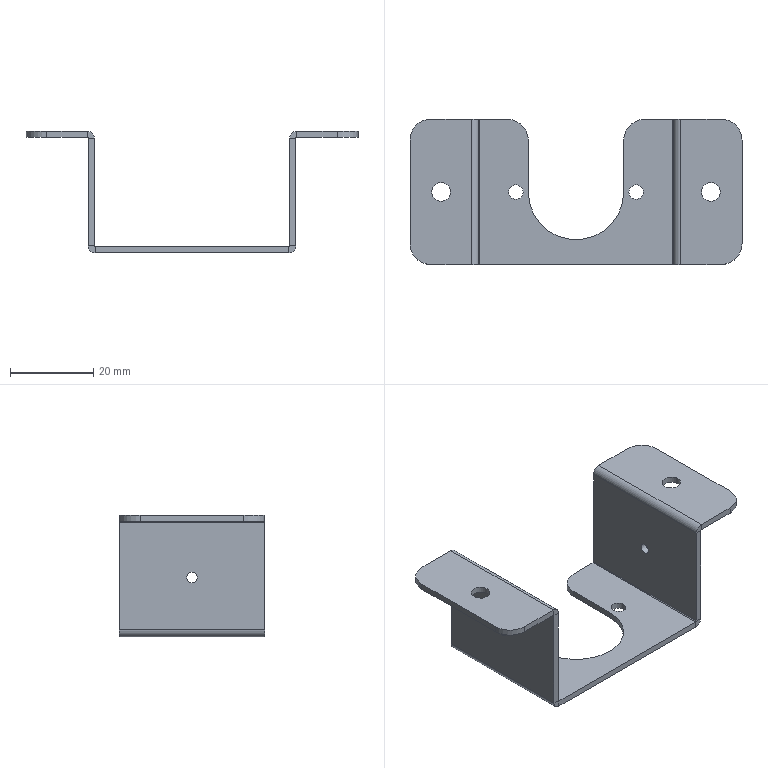Part | NX | 1 solid | 54 faces | box 80 x 35 x 29.3 mm | volume 5978 mm3 | plane 33 | cylinder 21 | commonest cylinder face diameters 10 x6 0.4 x4 3.4 x4 2.5 x2 3.5 x2 4.5 x2
STEP:
#1=CARTESIAN_POINT('',(-12.75,0.,-1.5));
#2=VERTEX_POINT('',#1);
#3=CARTESIAN_POINT('',(-14.5,0.,-1.5));
#4=DIRECTION('',(0.,0.,1.));
#5=DIRECTION('',(1.,0.,0.));
#6=AXIS2_PLACEMENT_3D('',#3,#4,#5);
#7=CIRCLE('',#6,1.75);
#8=EDGE_CURVE('',#2,#2,#7,.T.);
#9=ORIENTED_EDGE('',*,*,#8,.T.);
#10=EDGE_LOOP('',(#9));
#11=FACE_BOUND('',#10,.T.);
#12=CARTESIAN_POINT('',(12.75,0.,-1.5));
#13=VERTEX_POINT('',#12);
#14=CARTESIAN_POINT('',(14.5,0.,-1.5));
#15=DIRECTION('',(0.,0.,1.));
#16=DIRECTION('',(-1.,0.,0.));
#17=AXIS2_PLACEMENT_3D('',#14,#15,#16);
#18=CIRCLE('',#17,1.75);
#19=EDGE_CURVE('',#13,#13,#18,.T.);
#20=ORIENTED_EDGE('',*,*,#19,.T.);
#21=EDGE_LOOP('',(#20));
#22=FACE_BOUND('',#21,.T.);
#23=CARTESIAN_POINT('',(11.5,0.,-1.5));
#24=VERTEX_POINT('',#23);
#25=CARTESIAN_POINT('',(11.5,12.5,-1.5));
#26=VERTEX_POINT('',#25);
#27=CARTESIAN_POINT('',(11.5,0.,-1.5));
#28=DIRECTION('',(0.,1.,0.));
#29=VECTOR('',#28,1000.);
#30=LINE('',#27,#29);
#31=EDGE_CURVE('',#24,#26,#30,.T.);
#32=ORIENTED_EDGE('',*,*,#31,.T.);
#33=CARTESIAN_POINT('',(16.5,17.5,-1.5));
#34=VERTEX_POINT('',#33);
#35=CARTESIAN_POINT('',(16.5,12.5,-1.5));
#36=DIRECTION('',(0.,0.,-1.));
#37=DIRECTION('',(-1.,0.,0.));
#38=AXIS2_PLACEMENT_3D('',#35,#36,#37);
#39=CIRCLE('',#38,5.);
#40=EDGE_CURVE('',#26,#34,#39,.T.);
#41=ORIENTED_EDGE('',*,*,#40,.T.);
#42=CARTESIAN_POINT('',(23.3,17.5,-1.5));
#43=VERTEX_POINT('',#42);
#44=CARTESIAN_POINT('',(25.,17.5,-1.5));
#45=DIRECTION('',(-1.,0.,0.));
#46=VECTOR('',#45,1000.);
#47=LINE('',#44,#46);
#48=EDGE_CURVE('',#43,#34,#47,.T.);
#49=ORIENTED_EDGE('',*,*,#48,.F.);
#50=CARTESIAN_POINT('',(23.3,-17.5,-1.5));
#51=VERTEX_POINT('',#50);
#52=CARTESIAN_POINT('',(23.3,17.5,-1.5));
#53=DIRECTION('',(0.,1.,0.));
#54=VECTOR('',#53,1000.);
#55=LINE('',#52,#54);
#56=EDGE_CURVE('',#43,#51,#55,.F.);
#57=ORIENTED_EDGE('',*,*,#56,.T.);
#58=CARTESIAN_POINT('',(-23.3,-17.5,-1.5));
#59=VERTEX_POINT('',#58);
#60=CARTESIAN_POINT('',(25.,-17.5,-1.5));
#61=DIRECTION('',(1.,0.,0.));
#62=VECTOR('',#61,1000.);
#63=LINE('',#60,#62);
#64=EDGE_CURVE('',#59,#51,#63,.T.);
#65=ORIENTED_EDGE('',*,*,#64,.F.);
#66=CARTESIAN_POINT('',(-23.3,17.5,-1.5));
#67=VERTEX_POINT('',#66);
#68=CARTESIAN_POINT('',(-23.3,-17.5,-1.5));
#69=DIRECTION('',(0.,-1.,0.));
#70=VECTOR('',#69,1000.);
#71=LINE('',#68,#70);
#72=EDGE_CURVE('',#59,#67,#71,.F.);
#73=ORIENTED_EDGE('',*,*,#72,.T.);
#74=CARTESIAN_POINT('',(-16.5,17.5,-1.5));
#75=VERTEX_POINT('',#74);
#76=CARTESIAN_POINT('',(25.,17.5,-1.5));
#77=DIRECTION('',(-1.,0.,0.));
#78=VECTOR('',#77,1000.);
#79=LINE('',#76,#78);
#80=EDGE_CURVE('',#75,#67,#79,.T.);
#81=ORIENTED_EDGE('',*,*,#80,.F.);
#82=CARTESIAN_POINT('',(-11.5,12.5,-1.5));
#83=VERTEX_POINT('',#82);
#84=CARTESIAN_POINT('',(-16.5,12.5,-1.5));
#85=DIRECTION('',(0.,0.,-1.));
#86=DIRECTION('',(-1.,0.,0.));
#87=AXIS2_PLACEMENT_3D('',#84,#85,#86);
#88=CIRCLE('',#87,5.);
#89=EDGE_CURVE('',#75,#83,#88,.T.);
#90=ORIENTED_EDGE('',*,*,#89,.T.);
#91=CARTESIAN_POINT('',(-11.5,0.,-1.5));
#92=VERTEX_POINT('',#91);
#93=CARTESIAN_POINT('',(-11.5,0.,-1.5));
#94=DIRECTION('',(0.,1.,0.));
#95=VECTOR('',#94,1000.);
#96=LINE('',#93,#95);
#97=EDGE_CURVE('',#83,#92,#96,.F.);
#98=ORIENTED_EDGE('',*,*,#97,.T.);
#99=CARTESIAN_POINT('',(0.,0.,-1.5));
#100=DIRECTION('',(0.,0.,1.));
#101=DIRECTION('',(1.,0.,0.));
#102=AXIS2_PLACEMENT_3D('',#99,#100,#101);
#103=CIRCLE('',#102,11.5);
#104=EDGE_CURVE('',#92,#24,#103,.T.);
#105=ORIENTED_EDGE('',*,*,#104,.T.);
#106=EDGE_LOOP('',(#32,#41,#49,#57,#65,#73,#81,#90,#98,#105));
#107=FACE_BOUND('',#106,.T.);
#108=CARTESIAN_POINT('',(0.,0.,-1.5));
#109=DIRECTION('',(0.,0.,-1.));
#110=DIRECTION('',(-1.,0.,0.));
#111=AXIS2_PLACEMENT_3D('',#108,#109,#110);
#112=PLANE('',#111);
#113=ADVANCED_FACE('',(#11,#22,#107),#112,.T.);
#114=CARTESIAN_POINT('',(-12.75,0.,0.));
#115=VERTEX_POINT('',#114);
#116=CARTESIAN_POINT('',(-14.5,0.,0.));
#117=DIRECTION('',(0.,0.,1.));
#118=DIRECTION('',(1.,0.,0.));
#119=AXIS2_PLACEMENT_3D('',#116,#117,#118);
#120=CIRCLE('',#119,1.75);
#121=EDGE_CURVE('',#115,#115,#120,.T.);
#122=ORIENTED_EDGE('',*,*,#121,.F.);
#123=EDGE_LOOP('',(#122));
#124=FACE_BOUND('',#123,.T.);
#125=CARTESIAN_POINT('',(12.75,0.,0.));
#126=VERTEX_POINT('',#125);
#127=CARTESIAN_POINT('',(14.5,0.,0.));
#128=DIRECTION('',(0.,0.,1.));
#129=DIRECTION('',(-1.,0.,0.));
#130=AXIS2_PLACEMENT_3D('',#127,#128,#129);
#131=CIRCLE('',#130,1.75);
#132=EDGE_CURVE('',#126,#126,#131,.T.);
#133=ORIENTED_EDGE('',*,*,#132,.F.);
#134=EDGE_LOOP('',(#133));
#135=FACE_BOUND('',#134,.T.);
#136=CARTESIAN_POINT('',(23.3,17.5,0.));
#137=VERTEX_POINT('',#136);
#138=CARTESIAN_POINT('',(16.5,17.5,0.));
#139=VERTEX_POINT('',#138);
#140=CARTESIAN_POINT('',(25.,17.5,0.));
#141=DIRECTION('',(-1.,0.,0.));
#142=VECTOR('',#141,1000.);
#143=LINE('',#140,#142);
#144=EDGE_CURVE('',#137,#139,#143,.T.);
#145=ORIENTED_EDGE('',*,*,#144,.T.);
#146=CARTESIAN_POINT('',(11.5,12.5,0.));
#147=VERTEX_POINT('',#146);
#148=CARTESIAN_POINT('',(16.5,12.5,0.));
#149=DIRECTION('',(0.,0.,-1.));
#150=DIRECTION('',(-1.,0.,0.));
#151=AXIS2_PLACEMENT_3D('',#148,#149,#150);
#152=CIRCLE('',#151,5.);
#153=EDGE_CURVE('',#139,#147,#152,.F.);
#154=ORIENTED_EDGE('',*,*,#153,.T.);
#155=CARTESIAN_POINT('',(11.5,0.,0.));
#156=VERTEX_POINT('',#155);
#157=CARTESIAN_POINT('',(11.5,35.,0.));
#158=DIRECTION('',(0.,1.,0.));
#159=VECTOR('',#158,1000.);
#160=LINE('',#157,#159);
#161=EDGE_CURVE('',#156,#147,#160,.T.);
#162=ORIENTED_EDGE('',*,*,#161,.F.);
#163=CARTESIAN_POINT('',(-11.5,0.,0.));
#164=VERTEX_POINT('',#163);
#165=CARTESIAN_POINT('',(0.,0.,0.));
#166=DIRECTION('',(0.,0.,1.));
#167=DIRECTION('',(1.,0.,0.));
#168=AXIS2_PLACEMENT_3D('',#165,#166,#167);
#169=CIRCLE('',#168,11.5);
#170=EDGE_CURVE('',#164,#156,#169,.T.);
#171=ORIENTED_EDGE('',*,*,#170,.F.);
#172=CARTESIAN_POINT('',(-11.5,12.5,0.));
#173=VERTEX_POINT('',#172);
#174=CARTESIAN_POINT('',(-11.5,35.,0.));
#175=DIRECTION('',(0.,-1.,0.));
#176=VECTOR('',#175,1000.);
#177=LINE('',#174,#176);
#178=EDGE_CURVE('',#173,#164,#177,.T.);
#179=ORIENTED_EDGE('',*,*,#178,.F.);
#180=CARTESIAN_POINT('',(-16.5,17.5,0.));
#181=VERTEX_POINT('',#180);
#182=CARTESIAN_POINT('',(-16.5,12.5,0.));
#183=DIRECTION('',(0.,0.,-1.));
#184=DIRECTION('',(-1.,0.,0.));
#185=AXIS2_PLACEMENT_3D('',#182,#183,#184);
#186=CIRCLE('',#185,5.);
#187=EDGE_CURVE('',#173,#181,#186,.F.);
#188=ORIENTED_EDGE('',*,*,#187,.T.);
#189=CARTESIAN_POINT('',(-23.3,17.5,0.));
#190=VERTEX_POINT('',#189);
#191=CARTESIAN_POINT('',(25.,17.5,0.));
#192=DIRECTION('',(-1.,0.,0.));
#193=VECTOR('',#192,1000.);
#194=LINE('',#191,#193);
#195=EDGE_CURVE('',#181,#190,#194,.T.);
#196=ORIENTED_EDGE('',*,*,#195,.T.);
#197=CARTESIAN_POINT('',(-23.3,-17.5,0.));
#198=VERTEX_POINT('',#197);
#199=CARTESIAN_POINT('',(-23.3,-17.5,0.));
#200=DIRECTION('',(0.,-1.,0.));
#201=VECTOR('',#200,1000.);
#202=LINE('',#199,#201);
#203=EDGE_CURVE('',#198,#190,#202,.F.);
#204=ORIENTED_EDGE('',*,*,#203,.F.);
#205=CARTESIAN_POINT('',(23.3,-17.5,0.));
#206=VERTEX_POINT('',#205);
#207=CARTESIAN_POINT('',(25.,-17.5,0.));
#208=DIRECTION('',(1.,0.,0.));
#209=VECTOR('',#208,1000.);
#210=LINE('',#207,#209);
#211=EDGE_CURVE('',#198,#206,#210,.T.);
#212=ORIENTED_EDGE('',*,*,#211,.T.);
#213=CARTESIAN_POINT('',(23.3,17.5,0.));
#214=DIRECTION('',(0.,1.,0.));
#215=VECTOR('',#214,1000.);
#216=LINE('',#213,#215);
#217=EDGE_CURVE('',#137,#206,#216,.F.);
#218=ORIENTED_EDGE('',*,*,#217,.F.);
#219=EDGE_LOOP('',(#145,#154,#162,#171,#179,#188,#196,#204,#212,#218));
#220=FACE_BOUND('',#219,.T.);
#221=CARTESIAN_POINT('',(0.,0.,0.));
#222=DIRECTION('',(0.,0.,-1.));
#223=DIRECTION('',(-1.,0.,0.));
#224=AXIS2_PLACEMENT_3D('',#221,#222,#223);
#225=PLANE('',#224);
#226=ADVANCED_FACE('',(#124,#135,#220),#225,.F.);
#227=ORIENTED_EDGE('',*,*,#48,.T.);
#228=CARTESIAN_POINT('',(16.5,17.5,-1.5));
#229=DIRECTION('',(0.,0.,-1.));
#230=VECTOR('',#229,1000.);
#231=LINE('',#228,#230);
#232=EDGE_CURVE('',#34,#139,#231,.F.);
#233=ORIENTED_EDGE('',*,*,#232,.T.);
#234=ORIENTED_EDGE('',*,*,#144,.F.);
#235=CARTESIAN_POINT('',(23.3,17.5,0.));
#236=DIRECTION('',(0.,0.,-1.));
#237=VECTOR('',#236,1000.);
#238=LINE('',#235,#237);
#239=EDGE_CURVE('',#137,#43,#238,.T.);
#240=ORIENTED_EDGE('',*,*,#239,.T.);
#241=EDGE_LOOP('',(#227,#233,#234,#240));
#242=FACE_BOUND('',#241,.T.);
#243=CARTESIAN_POINT('',(25.,17.5,-1.5));
#244=DIRECTION('',(0.,1.,0.));
#245=DIRECTION('',(-1.,0.,0.));
#246=AXIS2_PLACEMENT_3D('',#243,#244,#245);
#247=PLANE('',#246);
#248=ADVANCED_FACE('',(#242),#247,.T.);
#249=ORIENTED_EDGE('',*,*,#195,.F.);
#250=CARTESIAN_POINT('',(-16.5,17.5,-1.5));
#251=DIRECTION('',(0.,0.,-1.));
#252=VECTOR('',#251,1000.);
#253=LINE('',#250,#252);
#254=EDGE_CURVE('',#181,#75,#253,.T.);
#255=ORIENTED_EDGE('',*,*,#254,.T.);
#256=ORIENTED_EDGE('',*,*,#80,.T.);
#257=CARTESIAN_POINT('',(-23.3,17.5,0.));
#258=DIRECTION('',(0.,0.,-1.));
#259=VECTOR('',#258,1000.);
#260=LINE('',#257,#259);
#261=EDGE_CURVE('',#190,#67,#260,.T.);
#262=ORIENTED_EDGE('',*,*,#261,.F.);
#263=EDGE_LOOP('',(#249,#255,#256,#262));
#264=FACE_BOUND('',#263,.T.);
#265=CARTESIAN_POINT('',(25.,17.5,-1.5));
#266=DIRECTION('',(0.,1.,0.));
#267=DIRECTION('',(-1.,0.,0.));
#268=AXIS2_PLACEMENT_3D('',#265,#266,#267);
#269=PLANE('',#268);
#270=ADVANCED_FACE('',(#264),#269,.T.);
#271=CARTESIAN_POINT('',(25.,-17.5,0.2));
#272=VERTEX_POINT('',#271);
#273=CARTESIAN_POINT('',(25.,-17.5,26.1));
#274=VERTEX_POINT('',#273);
#275=CARTESIAN_POINT('',(25.,-17.5,0.));
#276=DIRECTION('',(0.,0.,-1.));
#277=VECTOR('',#276,1000.);
#278=LINE('',#275,#277);
#279=EDGE_CURVE('',#272,#274,#278,.F.);
#280=ORIENTED_EDGE('',*,*,#279,.T.);
#281=CARTESIAN_POINT('',(23.5,-17.5,26.1));
#282=VERTEX_POINT('',#281);
#283=CARTESIAN_POINT('',(25.,-17.5,26.1));
#284=DIRECTION('',(-1.,0.,0.));
#285=VECTOR('',#284,1000.);
#286=LINE('',#283,#285);
#287=EDGE_CURVE('',#274,#282,#286,.T.);
#288=ORIENTED_EDGE('',*,*,#287,.T.);
#289=CARTESIAN_POINT('',(23.5,-17.5,0.2));
#290=VERTEX_POINT('',#289);
#291=CARTESIAN_POINT('',(23.5,-17.5,0.));
#292=DIRECTION('',(0.,0.,1.));
#293=VECTOR('',#292,1000.);
#294=LINE('',#291,#293);
#295=EDGE_CURVE('',#290,#282,#294,.T.);
#296=ORIENTED_EDGE('',*,*,#295,.F.);
#297=CARTESIAN_POINT('',(25.,-17.5,0.2));
#298=DIRECTION('',(1.,0.,0.));
#299=VECTOR('',#298,1000.);
#300=LINE('',#297,#299);
#301=EDGE_CURVE('',#290,#272,#300,.T.);
#302=ORIENTED_EDGE('',*,*,#301,.T.);
#303=EDGE_LOOP('',(#280,#288,#296,#302));
#304=FACE_BOUND('',#303,.T.);
#305=CARTESIAN_POINT('',(25.,-17.5,0.));
#306=DIRECTION('',(0.,-1.,0.));
#307=DIRECTION('',(1.,0.,0.));
#308=AXIS2_PLACEMENT_3D('',#305,#306,#307);
#309=PLANE('',#308);
#310=ADVANCED_FACE('',(#304),#309,.T.);
#311=CARTESIAN_POINT('',(25.,0.,14.05));
#312=VERTEX_POINT('',#311);
#313=CARTESIAN_POINT('',(25.,0.,12.8));
#314=DIRECTION('',(-1.,0.,0.));
#315=DIRECTION('',(0.,0.,1.));
#316=AXIS2_PLACEMENT_3D('',#313,#314,#315);
#317=CIRCLE('',#316,1.25);
#318=EDGE_CURVE('',#312,#312,#317,.T.);
#319=ORIENTED_EDGE('',*,*,#318,.T.);
#320=EDGE_LOOP('',(#319));
#321=FACE_BOUND('',#320,.T.);
#322=CARTESIAN_POINT('',(25.,17.5,26.1));
#323=VERTEX_POINT('',#322);
#324=CARTESIAN_POINT('',(25.,-17.5,26.1));
#325=DIRECTION('',(0.,-1.,0.));
#326=VECTOR('',#325,1000.);
#327=LINE('',#324,#326);
#328=EDGE_CURVE('',#274,#323,#327,.F.);
#329=ORIENTED_EDGE('',*,*,#328,.F.);
#330=ORIENTED_EDGE('',*,*,#279,.F.);
#331=CARTESIAN_POINT('',(25.,17.5,0.2));
#332=VERTEX_POINT('',#331);
#333=CARTESIAN_POINT('',(25.,-17.5,0.2));
#334=DIRECTION('',(0.,1.,0.));
#335=VECTOR('',#334,1000.);
#336=LINE('',#333,#335);
#337=EDGE_CURVE('',#332,#272,#336,.F.);
#338=ORIENTED_EDGE('',*,*,#337,.F.);
#339=CARTESIAN_POINT('',(25.,17.5,27.8));
#340=DIRECTION('',(0.,0.,1.));
#341=VECTOR('',#340,1000.);
#342=LINE('',#339,#341);
#343=EDGE_CURVE('',#323,#332,#342,.F.);
#344=ORIENTED_EDGE('',*,*,#343,.F.);
#345=EDGE_LOOP('',(#329,#330,#338,#344));
#346=FACE_BOUND('',#345,.T.);
#347=CARTESIAN_POINT('',(25.,0.,0.));
#348=DIRECTION('',(-1.,0.,0.));
#349=DIRECTION('',(0.,0.,1.));
#350=AXIS2_PLACEMENT_3D('',#347,#348,#349);
#351=PLANE('',#350);
#352=ADVANCED_FACE('',(#321,#346),#351,.F.);
#353=CARTESIAN_POINT('',(23.5,0.,14.05));
#354=VERTEX_POINT('',#353);
#355=CARTESIAN_POINT('',(23.5,0.,12.8));
#356=DIRECTION('',(-1.,0.,0.));
#357=DIRECTION('',(0.,0.,1.));
#358=AXIS2_PLACEMENT_3D('',#355,#356,#357);
#359=CIRCLE('',#358,1.25);
#360=EDGE_CURVE('',#354,#354,#359,.T.);
#361=ORIENTED_EDGE('',*,*,#360,.F.);
#362=EDGE_LOOP('',(#361));
#363=FACE_BOUND('',#362,.T.);
#364=ORIENTED_EDGE('',*,*,#295,.T.);
#365=CARTESIAN_POINT('',(23.5,17.5,26.1));
#366=VERTEX_POINT('',#365);
#367=CARTESIAN_POINT('',(23.5,-17.5,26.1));
#368=DIRECTION('',(0.,-1.,0.));
#369=VECTOR('',#368,1000.);
#370=LINE('',#367,#369);
#371=EDGE_CURVE('',#282,#366,#370,.F.);
#372=ORIENTED_EDGE('',*,*,#371,.T.);
#373=CARTESIAN_POINT('',(23.5,17.5,0.2));
#374=VERTEX_POINT('',#373);
#375=CARTESIAN_POINT('',(23.5,17.5,0.));
#376=DIRECTION('',(0.,0.,-1.));
#377=VECTOR('',#376,1000.);
#378=LINE('',#375,#377);
#379=EDGE_CURVE('',#366,#374,#378,.T.);
#380=ORIENTED_EDGE('',*,*,#379,.T.);
#381=CARTESIAN_POINT('',(23.5,-17.5,0.2));
#382=DIRECTION('',(0.,1.,0.));
#383=VECTOR('',#382,1000.);
#384=LINE('',#381,#383);
#385=EDGE_CURVE('',#290,#374,#384,.T.);
#386=ORIENTED_EDGE('',*,*,#385,.F.);
#387=EDGE_LOOP('',(#364,#372,#380,#386));
#388=FACE_BOUND('',#387,.T.);
#389=CARTESIAN_POINT('',(23.5,0.,0.));
#390=DIRECTION('',(-1.,0.,0.));
#391=DIRECTION('',(0.,0.,1.));
#392=AXIS2_PLACEMENT_3D('',#389,#390,#391);
#393=PLANE('',#392);
#394=ADVANCED_FACE('',(#363,#388),#393,.T.);
#395=CARTESIAN_POINT('',(-25.,17.5,0.2));
#396=VERTEX_POINT('',#395);
#397=CARTESIAN_POINT('',(-25.,17.5,26.1));
#398=VERTEX_POINT('',#397);
#399=CARTESIAN_POINT('',(-25.,17.5,27.8));
#400=DIRECTION('',(0.,0.,1.));
#401=VECTOR('',#400,1000.);
#402=LINE('',#399,#401);
#403=EDGE_CURVE('',#396,#398,#402,.T.);
#404=ORIENTED_EDGE('',*,*,#403,.T.);
#405=CARTESIAN_POINT('',(-23.5,17.5,26.1));
#406=VERTEX_POINT('',#405);
#407=CARTESIAN_POINT('',(-25.,17.5,26.1));
#408=DIRECTION('',(1.,0.,0.));
#409=VECTOR('',#408,1000.);
#410=LINE('',#407,#409);
#411=EDGE_CURVE('',#398,#406,#410,.T.);
#412=ORIENTED_EDGE('',*,*,#411,.T.);
#413=CARTESIAN_POINT('',(-23.5,17.5,0.2));
#414=VERTEX_POINT('',#413);
#415=CARTESIAN_POINT('',(-23.5,17.5,0.));
#416=DIRECTION('',(0.,0.,-1.));
#417=VECTOR('',#416,1000.);
#418=LINE('',#415,#417);
#419=EDGE_CURVE('',#414,#406,#418,.F.);
#420=ORIENTED_EDGE('',*,*,#419,.F.);
#421=CARTESIAN_POINT('',(-25.,17.5,0.2));
#422=DIRECTION('',(-1.,0.,0.));
#423=VECTOR('',#422,1000.);
#424=LINE('',#421,#423);
#425=EDGE_CURVE('',#414,#396,#424,.T.);
#426=ORIENTED_EDGE('',*,*,#425,.T.);
#427=EDGE_LOOP('',(#404,#412,#420,#426));
#428=FACE_BOUND('',#427,.T.);
#429=CARTESIAN_POINT('',(-25.,17.5,27.8));
#430=DIRECTION('',(0.,1.,0.));
#431=DIRECTION('',(-1.,0.,0.));
#432=AXIS2_PLACEMENT_3D('',#429,#430,#431);
#433=PLANE('',#432);
#434=ADVANCED_FACE('',(#428),#433,.T.);
#435=CARTESIAN_POINT('',(-25.,0.,14.05));
#436=VERTEX_POINT('',#435);
#437=CARTESIAN_POINT('',(-25.,0.,12.8));
#438=DIRECTION('',(-1.,0.,0.));
#439=DIRECTION('',(0.,0.,1.));
#440=AXIS2_PLACEMENT_3D('',#437,#438,#439);
#441=CIRCLE('',#440,1.25);
#442=EDGE_CURVE('',#436,#436,#441,.T.);
#443=ORIENTED_EDGE('',*,*,#442,.F.);
#444=EDGE_LOOP('',(#443));
#445=FACE_BOUND('',#444,.T.);
#446=CARTESIAN_POINT('',(-25.,-17.5,26.1));
#447=VERTEX_POINT('',#446);
#448=CARTESIAN_POINT('',(-25.,-17.5,0.2));
#449=VERTEX_POINT('',#448);
#450=CARTESIAN_POINT('',(-25.,-17.5,0.));
#451=DIRECTION('',(0.,0.,-1.));
#452=VECTOR('',#451,1000.);
#453=LINE('',#450,#452);
#454=EDGE_CURVE('',#447,#449,#453,.T.);
#455=ORIENTED_EDGE('',*,*,#454,.F.);
#456=CARTESIAN_POINT('',(-25.,17.5,26.1));
#457=DIRECTION('',(0.,1.,0.));
#458=VECTOR('',#457,1000.);
#459=LINE('',#456,#458);
#460=EDGE_CURVE('',#398,#447,#459,.F.);
#461=ORIENTED_EDGE('',*,*,#460,.F.);
#462=ORIENTED_EDGE('',*,*,#403,.F.);
#463=CARTESIAN_POINT('',(-25.,0.,0.2));
#464=DIRECTION('',(0.,-1.,0.));
#465=VECTOR('',#464,1000.);
#466=LINE('',#463,#465);
#467=EDGE_CURVE('',#396,#449,#466,.T.);
#468=ORIENTED_EDGE('',*,*,#467,.T.);
#469=EDGE_LOOP('',(#455,#461,#462,#468));
#470=FACE_BOUND('',#469,.T.);
#471=CARTESIAN_POINT('',(-25.,0.,0.));
#472=DIRECTION('',(-1.,0.,0.));
#473=DIRECTION('',(0.,0.,1.));
#474=AXIS2_PLACEMENT_3D('',#471,#472,#473);
#475=PLANE('',#474);
#476=ADVANCED_FACE('',(#445,#470),#475,.T.);
#477=CARTESIAN_POINT('',(-23.5,0.,14.05));
#478=VERTEX_POINT('',#477);
#479=CARTESIAN_POINT('',(-23.5,0.,12.8));
#480=DIRECTION('',(-1.,0.,0.));
#481=DIRECTION('',(0.,0.,1.));
#482=AXIS2_PLACEMENT_3D('',#479,#480,#481);
#483=CIRCLE('',#482,1.25);
#484=EDGE_CURVE('',#478,#478,#483,.T.);
#485=ORIENTED_EDGE('',*,*,#484,.T.);
#486=EDGE_LOOP('',(#485));
#487=FACE_BOUND('',#486,.T.);
#488=CARTESIAN_POINT('',(-23.5,-17.5,26.1));
#489=VERTEX_POINT('',#488);
#490=CARTESIAN_POINT('',(-23.5,17.5,26.1));
#491=DIRECTION('',(0.,1.,0.));
#492=VECTOR('',#491,1000.);
#493=LINE('',#490,#492);
#494=EDGE_CURVE('',#406,#489,#493,.F.);
#495=ORIENTED_EDGE('',*,*,#494,.T.);
#496=CARTESIAN_POINT('',(-23.5,-17.5,0.2));
#497=VERTEX_POINT('',#496);
#498=CARTESIAN_POINT('',(-23.5,-17.5,0.));
#499=DIRECTION('',(0.,0.,1.));
#500=VECTOR('',#499,1000.);
#501=LINE('',#498,#500);
#502=EDGE_CURVE('',#489,#497,#501,.F.);
#503=ORIENTED_EDGE('',*,*,#502,.T.);
#504=CARTESIAN_POINT('',(-23.5,17.5,0.2));
#505=DIRECTION('',(0.,1.,0.));
#506=VECTOR('',#505,1000.);
#507=LINE('',#504,#506);
#508=EDGE_CURVE('',#414,#497,#507,.F.);
#509=ORIENTED_EDGE('',*,*,#508,.F.);
#510=ORIENTED_EDGE('',*,*,#419,.T.);
#511=EDGE_LOOP('',(#495,#503,#509,#510));
#512=FACE_BOUND('',#511,.T.);
#513=CARTESIAN_POINT('',(-23.5,0.,0.));
#514=DIRECTION('',(-1.,0.,0.));
#515=DIRECTION('',(0.,0.,1.));
#516=AXIS2_PLACEMENT_3D('',#513,#514,#515);
#517=PLANE('',#516);
#518=ADVANCED_FACE('',(#487,#512),#517,.F.);
#519=CARTESIAN_POINT('',(23.3,-17.5,0.));
#520=DIRECTION('',(0.,0.,-1.));
#521=VECTOR('',#520,1000.);
#522=LINE('',#519,#521);
#523=EDGE_CURVE('',#206,#51,#522,.T.);
#524=ORIENTED_EDGE('',*,*,#523,.F.);
#525=ORIENTED_EDGE('',*,*,#211,.F.);
#526=CARTESIAN_POINT('',(-23.3,-17.5,0.));
#527=DIRECTION('',(0.,0.,-1.));
#528=VECTOR('',#527,1000.);
#529=LINE('',#526,#528);
#530=EDGE_CURVE('',#198,#59,#529,.T.);
#531=ORIENTED_EDGE('',*,*,#530,.T.);
#532=ORIENTED_EDGE('',*,*,#64,.T.);
#533=EDGE_LOOP('',(#524,#525,#531,#532));
#534=FACE_BOUND('',#533,.T.);
#535=CARTESIAN_POINT('',(25.,-17.5,-1.5));
#536=DIRECTION('',(0.,-1.,0.));
#537=DIRECTION('',(1.,0.,0.));
#538=AXIS2_PLACEMENT_3D('',#535,#536,#537);
#539=PLANE('',#538);
#540=ADVANCED_FACE('',(#534),#539,.T.);
#541=ORIENTED_EDGE('',*,*,#425,.F.);
#542=CARTESIAN_POINT('',(-23.3,17.5,0.2));
#543=DIRECTION('',(0.,-1.,0.));
#544=DIRECTION('',(0.,0.,-1.));
#545=AXIS2_PLACEMENT_3D('',#542,#543,#544);
#546=CIRCLE('',#545,0.2);
#547=EDGE_CURVE('',#190,#414,#546,.F.);
#548=ORIENTED_EDGE('',*,*,#547,.F.);
#549=ORIENTED_EDGE('',*,*,#261,.T.);
#550=CARTESIAN_POINT('',(-23.3,17.5,0.2));
#551=DIRECTION('',(0.,-1.,0.));
#552=DIRECTION('',(0.,0.,-1.));
#553=AXIS2_PLACEMENT_3D('',#550,#551,#552);
#554=CIRCLE('',#553,1.7);
#555=EDGE_CURVE('',#67,#396,#554,.F.);
#556=ORIENTED_EDGE('',*,*,#555,.T.);
#557=EDGE_LOOP('',(#541,#548,#549,#556));
#558=FACE_BOUND('',#557,.T.);
#559=CARTESIAN_POINT('',(-23.3,17.5,0.2));
#560=DIRECTION('',(0.,1.,0.));
#561=DIRECTION('',(0.,0.,1.));
#562=AXIS2_PLACEMENT_3D('',#559,#560,#561);
#563=PLANE('',#562);
#564=ADVANCED_FACE('',(#558),#563,.T.);
#565=CARTESIAN_POINT('',(-23.3,-17.5,0.2));
#566=DIRECTION('',(0.,-1.,0.));
#567=DIRECTION('',(0.,0.,-1.));
#568=AXIS2_PLACEMENT_3D('',#565,#566,#567);
#569=CIRCLE('',#568,0.2);
#570=EDGE_CURVE('',#497,#198,#569,.T.);
#571=ORIENTED_EDGE('',*,*,#570,.F.);
#572=CARTESIAN_POINT('',(-23.5,-17.5,0.2));
#573=DIRECTION('',(-1.,0.,0.));
#574=VECTOR('',#573,1000.);
#575=LINE('',#572,#574);
#576=EDGE_CURVE('',#497,#449,#575,.T.);
#577=ORIENTED_EDGE('',*,*,#576,.T.);
#578=CARTESIAN_POINT('',(-23.3,-17.5,0.2));
#579=DIRECTION('',(0.,-1.,0.));
#580=DIRECTION('',(0.,0.,-1.));
#581=AXIS2_PLACEMENT_3D('',#578,#579,#580);
#582=CIRCLE('',#581,1.7);
#583=EDGE_CURVE('',#449,#59,#582,.T.);
#584=ORIENTED_EDGE('',*,*,#583,.T.);
#585=ORIENTED_EDGE('',*,*,#530,.F.);
#586=EDGE_LOOP('',(#571,#577,#584,#585));
#587=FACE_BOUND('',#586,.T.);
#588=CARTESIAN_POINT('',(-23.3,-17.5,0.2));
#589=DIRECTION('',(0.,1.,0.));
#590=DIRECTION('',(0.,0.,1.));
#591=AXIS2_PLACEMENT_3D('',#588,#589,#590);
#592=PLANE('',#591);
#593=ADVANCED_FACE('',(#587),#592,.F.);
#594=ORIENTED_EDGE('',*,*,#72,.F.);
#595=ORIENTED_EDGE('',*,*,#583,.F.);
#596=ORIENTED_EDGE('',*,*,#467,.F.);
#597=ORIENTED_EDGE('',*,*,#555,.F.);
#598=EDGE_LOOP('',(#594,#595,#596,#597));
#599=FACE_BOUND('',#598,.T.);
#600=CARTESIAN_POINT('',(-23.3,-17.5,0.2));
#601=DIRECTION('',(0.,-1.,0.));
#602=DIRECTION('',(-1.,0.,0.));
#603=AXIS2_PLACEMENT_3D('',#600,#601,#602);
#604=CYLINDRICAL_SURFACE('',#603,1.7);
#605=ADVANCED_FACE('',(#599),#604,.T.);
#606=ORIENTED_EDGE('',*,*,#203,.T.);
#607=ORIENTED_EDGE('',*,*,#547,.T.);
#608=ORIENTED_EDGE('',*,*,#508,.T.);
#609=ORIENTED_EDGE('',*,*,#570,.T.);
#610=EDGE_LOOP('',(#606,#607,#608,#609));
#611=FACE_BOUND('',#610,.T.);
#612=CARTESIAN_POINT('',(-23.3,-17.5,0.2));
#613=DIRECTION('',(0.,-1.,0.));
#614=DIRECTION('',(-1.,0.,0.));
#615=AXIS2_PLACEMENT_3D('',#612,#613,#614);
#616=CYLINDRICAL_SURFACE('',#615,0.2);
#617=ADVANCED_FACE('',(#611),#616,.F.);
#618=CARTESIAN_POINT('',(-25.,-17.5,26.1));
#619=DIRECTION('',(1.,0.,0.));
#620=VECTOR('',#619,1000.);
#621=LINE('',#618,#620);
#622=EDGE_CURVE('',#447,#489,#621,.T.);
#623=ORIENTED_EDGE('',*,*,#622,.F.);
#624=ORIENTED_EDGE('',*,*,#454,.T.);
#625=ORIENTED_EDGE('',*,*,#576,.F.);
#626=ORIENTED_EDGE('',*,*,#502,.F.);
#627=EDGE_LOOP('',(#623,#624,#625,#626));
#628=FACE_BOUND('',#627,.T.);
#629=CARTESIAN_POINT('',(-25.,-17.5,0.));
#630=DIRECTION('',(0.,-1.,0.));
#631=DIRECTION('',(1.,0.,0.));
#632=AXIS2_PLACEMENT_3D('',#629,#630,#631);
#633=PLANE('',#632);
#634=ADVANCED_FACE('',(#628),#633,.T.);
#635=ORIENTED_EDGE('',*,*,#301,.F.);
#636=CARTESIAN_POINT('',(23.3,-17.5,0.2));
#637=DIRECTION('',(0.,1.,0.));
#638=DIRECTION('',(0.,0.,1.));
#639=AXIS2_PLACEMENT_3D('',#636,#637,#638);
#640=CIRCLE('',#639,0.2);
#641=EDGE_CURVE('',#206,#290,#640,.F.);
#642=ORIENTED_EDGE('',*,*,#641,.F.);
#643=ORIENTED_EDGE('',*,*,#523,.T.);
#644=CARTESIAN_POINT('',(23.3,-17.5,0.2));
#645=DIRECTION('',(0.,1.,0.));
#646=DIRECTION('',(0.,0.,1.));
#647=AXIS2_PLACEMENT_3D('',#644,#645,#646);
#648=CIRCLE('',#647,1.7);
#649=EDGE_CURVE('',#51,#272,#648,.F.);
#650=ORIENTED_EDGE('',*,*,#649,.T.);
#651=EDGE_LOOP('',(#635,#642,#643,#650));
#652=FACE_BOUND('',#651,.T.);
#653=CARTESIAN_POINT('',(23.3,-17.5,0.2));
#654=DIRECTION('',(0.,-1.,0.));
#655=DIRECTION('',(0.,0.,-1.));
#656=AXIS2_PLACEMENT_3D('',#653,#654,#655);
#657=PLANE('',#656);
#658=ADVANCED_FACE('',(#652),#657,.T.);
#659=CARTESIAN_POINT('',(23.3,17.5,0.2));
#660=DIRECTION('',(0.,1.,0.));
#661=DIRECTION('',(0.,0.,1.));
#662=AXIS2_PLACEMENT_3D('',#659,#660,#661);
#663=CIRCLE('',#662,0.2);
#664=EDGE_CURVE('',#374,#137,#663,.T.);
#665=ORIENTED_EDGE('',*,*,#664,.F.);
#666=CARTESIAN_POINT('',(23.5,17.5,0.2));
#667=DIRECTION('',(1.,0.,0.));
#668=VECTOR('',#667,1000.);
#669=LINE('',#666,#668);
#670=EDGE_CURVE('',#374,#332,#669,.T.);
#671=ORIENTED_EDGE('',*,*,#670,.T.);
#672=CARTESIAN_POINT('',(23.3,17.5,0.2));
#673=DIRECTION('',(0.,1.,0.));
#674=DIRECTION('',(0.,0.,1.));
#675=AXIS2_PLACEMENT_3D('',#672,#673,#674);
#676=CIRCLE('',#675,1.7);
#677=EDGE_CURVE('',#332,#43,#676,.T.);
#678=ORIENTED_EDGE('',*,*,#677,.T.);
#679=ORIENTED_EDGE('',*,*,#239,.F.);
#680=EDGE_LOOP('',(#665,#671,#678,#679));
#681=FACE_BOUND('',#680,.T.);
#682=CARTESIAN_POINT('',(23.3,17.5,0.2));
#683=DIRECTION('',(0.,-1.,0.));
#684=DIRECTION('',(0.,0.,-1.));
#685=AXIS2_PLACEMENT_3D('',#682,#683,#684);
#686=PLANE('',#685);
#687=ADVANCED_FACE('',(#681),#686,.F.);
#688=ORIENTED_EDGE('',*,*,#56,.F.);
#689=ORIENTED_EDGE('',*,*,#677,.F.);
#690=ORIENTED_EDGE('',*,*,#337,.T.);
#691=ORIENTED_EDGE('',*,*,#649,.F.);
#692=EDGE_LOOP('',(#688,#689,#690,#691));
#693=FACE_BOUND('',#692,.T.);
#694=CARTESIAN_POINT('',(23.3,17.5,0.2));
#695=DIRECTION('',(0.,1.,0.));
#696=DIRECTION('',(1.,0.,0.));
#697=AXIS2_PLACEMENT_3D('',#694,#695,#696);
#698=CYLINDRICAL_SURFACE('',#697,1.7);
#699=ADVANCED_FACE('',(#693),#698,.T.);
#700=ORIENTED_EDGE('',*,*,#217,.T.);
#701=ORIENTED_EDGE('',*,*,#641,.T.);
#702=ORIENTED_EDGE('',*,*,#385,.T.);
#703=ORIENTED_EDGE('',*,*,#664,.T.);
#704=EDGE_LOOP('',(#700,#701,#702,#703));
#705=FACE_BOUND('',#704,.T.);
#706=CARTESIAN_POINT('',(23.3,17.5,0.2));
#707=DIRECTION('',(0.,1.,0.));
#708=DIRECTION('',(1.,0.,0.));
#709=AXIS2_PLACEMENT_3D('',#706,#707,#708);
#710=CYLINDRICAL_SURFACE('',#709,0.2);
#711=ADVANCED_FACE('',(#705),#710,.F.);
#712=CARTESIAN_POINT('',(25.,17.5,26.1));
#713=DIRECTION('',(-1.,0.,0.));
#714=VECTOR('',#713,1000.);
#715=LINE('',#712,#714);
#716=EDGE_CURVE('',#323,#366,#715,.T.);
#717=ORIENTED_EDGE('',*,*,#716,.F.);
#718=ORIENTED_EDGE('',*,*,#343,.T.);
#719=ORIENTED_EDGE('',*,*,#670,.F.);
#720=ORIENTED_EDGE('',*,*,#379,.F.);
#721=EDGE_LOOP('',(#717,#718,#719,#720));
#722=FACE_BOUND('',#721,.T.);
#723=CARTESIAN_POINT('',(25.,17.5,27.8));
#724=DIRECTION('',(0.,1.,0.));
#725=DIRECTION('',(0.,0.,1.));
#726=AXIS2_PLACEMENT_3D('',#723,#724,#725);
#727=PLANE('',#726);
#728=ADVANCED_FACE('',(#722),#727,.T.);
#729=CARTESIAN_POINT('',(-25.2,-17.5,26.3));
#730=VERTEX_POINT('',#729);
#731=CARTESIAN_POINT('',(-25.2,-17.5,27.8));
#732=VERTEX_POINT('',#731);
#733=CARTESIAN_POINT('',(-25.2,-17.5,27.8));
#734=DIRECTION('',(0.,0.,1.));
#735=VECTOR('',#734,1000.);
#736=LINE('',#733,#735);
#737=EDGE_CURVE('',#730,#732,#736,.T.);
#738=ORIENTED_EDGE('',*,*,#737,.F.);
#739=CARTESIAN_POINT('',(-25.2,-17.5,26.1));
#740=DIRECTION('',(0.,1.,0.));
#741=DIRECTION('',(0.,0.,1.));
#742=AXIS2_PLACEMENT_3D('',#739,#740,#741);
#743=CIRCLE('',#742,0.2);
#744=EDGE_CURVE('',#447,#730,#743,.F.);
#745=ORIENTED_EDGE('',*,*,#744,.F.);
#746=ORIENTED_EDGE('',*,*,#622,.T.);
#747=CARTESIAN_POINT('',(-25.2,-17.5,26.1));
#748=DIRECTION('',(0.,1.,0.));
#749=DIRECTION('',(0.,0.,1.));
#750=AXIS2_PLACEMENT_3D('',#747,#748,#749);
#751=CIRCLE('',#750,1.7);
#752=EDGE_CURVE('',#489,#732,#751,.F.);
#753=ORIENTED_EDGE('',*,*,#752,.T.);
#754=EDGE_LOOP('',(#738,#745,#746,#753));
#755=FACE_BOUND('',#754,.T.);
#756=CARTESIAN_POINT('',(-25.2,-17.5,26.1));
#757=DIRECTION('',(0.,-1.,0.));
#758=DIRECTION('',(0.,0.,-1.));
#759=AXIS2_PLACEMENT_3D('',#756,#757,#758);
#760=PLANE('',#759);
#761=ADVANCED_FACE('',(#755),#760,.T.);
#762=CARTESIAN_POINT('',(-25.2,17.5,26.3));
#763=VERTEX_POINT('',#762);
#764=CARTESIAN_POINT('',(-25.2,17.5,26.1));
#765=DIRECTION('',(0.,1.,0.));
#766=DIRECTION('',(0.,0.,1.));
#767=AXIS2_PLACEMENT_3D('',#764,#765,#766);
#768=CIRCLE('',#767,0.2);
#769=EDGE_CURVE('',#763,#398,#768,.T.);
#770=ORIENTED_EDGE('',*,*,#769,.F.);
#771=CARTESIAN_POINT('',(-25.2,17.5,27.8));
#772=VERTEX_POINT('',#771);
#773=CARTESIAN_POINT('',(-25.2,17.5,26.3));
#774=DIRECTION('',(0.,0.,1.));
#775=VECTOR('',#774,1000.);
#776=LINE('',#773,#775);
#777=EDGE_CURVE('',#763,#772,#776,.T.);
#778=ORIENTED_EDGE('',*,*,#777,.T.);
#779=CARTESIAN_POINT('',(-25.2,17.5,26.1));
#780=DIRECTION('',(0.,1.,0.));
#781=DIRECTION('',(0.,0.,1.));
#782=AXIS2_PLACEMENT_3D('',#779,#780,#781);
#783=CIRCLE('',#782,1.7);
#784=EDGE_CURVE('',#772,#406,#783,.T.);
#785=ORIENTED_EDGE('',*,*,#784,.T.);
#786=ORIENTED_EDGE('',*,*,#411,.F.);
#787=EDGE_LOOP('',(#770,#778,#785,#786));
#788=FACE_BOUND('',#787,.T.);
#789=CARTESIAN_POINT('',(-25.2,17.5,26.1));
#790=DIRECTION('',(0.,-1.,0.));
#791=DIRECTION('',(0.,0.,-1.));
#792=AXIS2_PLACEMENT_3D('',#789,#790,#791);
#793=PLANE('',#792);
#794=ADVANCED_FACE('',(#788),#793,.F.);
#795=ORIENTED_EDGE('',*,*,#494,.F.);
#796=ORIENTED_EDGE('',*,*,#784,.F.);
#797=CARTESIAN_POINT('',(-25.2,0.,27.8));
#798=DIRECTION('',(0.,1.,0.));
#799=VECTOR('',#798,1000.);
#800=LINE('',#797,#799);
#801=EDGE_CURVE('',#732,#772,#800,.T.);
#802=ORIENTED_EDGE('',*,*,#801,.F.);
#803=ORIENTED_EDGE('',*,*,#752,.F.);
#804=EDGE_LOOP('',(#795,#796,#802,#803));
#805=FACE_BOUND('',#804,.T.);
#806=CARTESIAN_POINT('',(-25.2,17.5,26.1));
#807=DIRECTION('',(0.,1.,0.));
#808=DIRECTION('',(0.,0.,1.));
#809=AXIS2_PLACEMENT_3D('',#806,#807,#808);
#810=CYLINDRICAL_SURFACE('',#809,1.7);
#811=ADVANCED_FACE('',(#805),#810,.T.);
#812=ORIENTED_EDGE('',*,*,#460,.T.);
#813=ORIENTED_EDGE('',*,*,#744,.T.);
#814=CARTESIAN_POINT('',(-25.2,-17.5,26.3));
#815=DIRECTION('',(0.,-1.,0.));
#816=VECTOR('',#815,1000.);
#817=LINE('',#814,#816);
#818=EDGE_CURVE('',#730,#763,#817,.F.);
#819=ORIENTED_EDGE('',*,*,#818,.T.);
#820=ORIENTED_EDGE('',*,*,#769,.T.);
#821=EDGE_LOOP('',(#812,#813,#819,#820));
#822=FACE_BOUND('',#821,.T.);
#823=CARTESIAN_POINT('',(-25.2,17.5,26.1));
#824=DIRECTION('',(0.,1.,0.));
#825=DIRECTION('',(0.,0.,1.));
#826=AXIS2_PLACEMENT_3D('',#823,#824,#825);
#827=CYLINDRICAL_SURFACE('',#826,0.2);
#828=ADVANCED_FACE('',(#822),#827,.F.);
#829=CARTESIAN_POINT('',(-35.,17.5,26.3));
#830=VERTEX_POINT('',#829);
#831=CARTESIAN_POINT('',(0.,17.5,26.3));
#832=DIRECTION('',(-1.,0.,0.));
#833=VECTOR('',#832,1000.);
#834=LINE('',#831,#833);
#835=EDGE_CURVE('',#830,#763,#834,.F.);
#836=ORIENTED_EDGE('',*,*,#835,.F.);
#837=CARTESIAN_POINT('',(-35.,17.5,27.8));
#838=VERTEX_POINT('',#837);
#839=CARTESIAN_POINT('',(-35.,17.5,27.8));
#840=DIRECTION('',(0.,0.,-1.));
#841=VECTOR('',#840,1000.);
#842=LINE('',#839,#841);
#843=EDGE_CURVE('',#830,#838,#842,.F.);
#844=ORIENTED_EDGE('',*,*,#843,.T.);
#845=CARTESIAN_POINT('',(-25.,17.5,27.8));
#846=DIRECTION('',(1.,0.,0.));
#847=VECTOR('',#846,1000.);
#848=LINE('',#845,#847);
#849=EDGE_CURVE('',#838,#772,#848,.T.);
#850=ORIENTED_EDGE('',*,*,#849,.T.);
#851=ORIENTED_EDGE('',*,*,#777,.F.);
#852=EDGE_LOOP('',(#836,#844,#850,#851));
#853=FACE_BOUND('',#852,.T.);
#854=CARTESIAN_POINT('',(-25.,17.5,27.8));
#855=DIRECTION('',(0.,1.,0.));
#856=DIRECTION('',(-1.,0.,0.));
#857=AXIS2_PLACEMENT_3D('',#854,#855,#856);
#858=PLANE('',#857);
#859=ADVANCED_FACE('',(#853),#858,.T.);
#860=CARTESIAN_POINT('',(-35.,-17.5,27.8));
#861=VERTEX_POINT('',#860);
#862=CARTESIAN_POINT('',(-40.,-17.5,27.8));
#863=DIRECTION('',(-1.,0.,0.));
#864=VECTOR('',#863,1000.);
#865=LINE('',#862,#864);
#866=EDGE_CURVE('',#732,#861,#865,.T.);
#867=ORIENTED_EDGE('',*,*,#866,.T.);
#868=CARTESIAN_POINT('',(-35.,-17.5,26.3));
#869=VERTEX_POINT('',#868);
#870=CARTESIAN_POINT('',(-35.,-17.5,27.8));
#871=DIRECTION('',(0.,0.,-1.));
#872=VECTOR('',#871,1000.);
#873=LINE('',#870,#872);
#874=EDGE_CURVE('',#861,#869,#873,.T.);
#875=ORIENTED_EDGE('',*,*,#874,.T.);
#876=CARTESIAN_POINT('',(0.,-17.5,26.3));
#877=DIRECTION('',(1.,0.,0.));
#878=VECTOR('',#877,1000.);
#879=LINE('',#876,#878);
#880=EDGE_CURVE('',#730,#869,#879,.F.);
#881=ORIENTED_EDGE('',*,*,#880,.F.);
#882=ORIENTED_EDGE('',*,*,#737,.T.);
#883=EDGE_LOOP('',(#867,#875,#881,#882));
#884=FACE_BOUND('',#883,.T.);
#885=CARTESIAN_POINT('',(-40.,-17.5,27.8));
#886=DIRECTION('',(0.,-1.,0.));
#887=DIRECTION('',(0.,0.,-1.));
#888=AXIS2_PLACEMENT_3D('',#885,#886,#887);
#889=PLANE('',#888);
#890=ADVANCED_FACE('',(#884),#889,.T.);
#891=CARTESIAN_POINT('',(-30.25,0.,27.8));
#892=VERTEX_POINT('',#891);
#893=CARTESIAN_POINT('',(-32.5,0.,27.8));
#894=DIRECTION('',(0.,0.,1.));
#895=DIRECTION('',(1.,0.,0.));
#896=AXIS2_PLACEMENT_3D('',#893,#894,#895);
#897=CIRCLE('',#896,2.25);
#898=EDGE_CURVE('',#892,#892,#897,.T.);
#899=ORIENTED_EDGE('',*,*,#898,.F.);
#900=EDGE_LOOP('',(#899));
#901=FACE_BOUND('',#900,.T.);
#902=ORIENTED_EDGE('',*,*,#849,.F.);
#903=CARTESIAN_POINT('',(-40.,12.5,27.8));
#904=VERTEX_POINT('',#903);
#905=CARTESIAN_POINT('',(-35.,12.5,27.8));
#906=DIRECTION('',(0.,0.,1.));
#907=DIRECTION('',(1.,0.,0.));
#908=AXIS2_PLACEMENT_3D('',#905,#906,#907);
#909=CIRCLE('',#908,5.);
#910=EDGE_CURVE('',#838,#904,#909,.T.);
#911=ORIENTED_EDGE('',*,*,#910,.T.);
#912=CARTESIAN_POINT('',(-40.,-12.5,27.8));
#913=VERTEX_POINT('',#912);
#914=CARTESIAN_POINT('',(-40.,17.5,27.8));
#915=DIRECTION('',(0.,1.,0.));
#916=VECTOR('',#915,1000.);
#917=LINE('',#914,#916);
#918=EDGE_CURVE('',#913,#904,#917,.T.);
#919=ORIENTED_EDGE('',*,*,#918,.F.);
#920=CARTESIAN_POINT('',(-35.,-12.5,27.8));
#921=DIRECTION('',(0.,0.,1.));
#922=DIRECTION('',(1.,0.,0.));
#923=AXIS2_PLACEMENT_3D('',#920,#921,#922);
#924=CIRCLE('',#923,5.);
#925=EDGE_CURVE('',#913,#861,#924,.T.);
#926=ORIENTED_EDGE('',*,*,#925,.T.);
#927=ORIENTED_EDGE('',*,*,#866,.F.);
#928=ORIENTED_EDGE('',*,*,#801,.T.);
#929=EDGE_LOOP('',(#902,#911,#919,#926,#927,#928));
#930=FACE_BOUND('',#929,.T.);
#931=CARTESIAN_POINT('',(0.,0.,27.8));
#932=DIRECTION('',(0.,0.,1.));
#933=DIRECTION('',(1.,0.,0.));
#934=AXIS2_PLACEMENT_3D('',#931,#932,#933);
#935=PLANE('',#934);
#936=ADVANCED_FACE('',(#901,#930),#935,.T.);
#937=CARTESIAN_POINT('',(-30.25,0.,26.3));
#938=VERTEX_POINT('',#937);
#939=CARTESIAN_POINT('',(-32.5,0.,26.3));
#940=DIRECTION('',(0.,0.,1.));
#941=DIRECTION('',(1.,0.,0.));
#942=AXIS2_PLACEMENT_3D('',#939,#940,#941);
#943=CIRCLE('',#942,2.25);
#944=EDGE_CURVE('',#938,#938,#943,.T.);
#945=ORIENTED_EDGE('',*,*,#944,.T.);
#946=EDGE_LOOP('',(#945));
#947=FACE_BOUND('',#946,.T.);
#948=CARTESIAN_POINT('',(-40.,-12.5,26.3));
#949=VERTEX_POINT('',#948);
#950=CARTESIAN_POINT('',(-40.,12.5,26.3));
#951=VERTEX_POINT('',#950);
#952=CARTESIAN_POINT('',(-40.,0.,26.3));
#953=DIRECTION('',(0.,-1.,0.));
#954=VECTOR('',#953,1000.);
#955=LINE('',#952,#954);
#956=EDGE_CURVE('',#949,#951,#955,.F.);
#957=ORIENTED_EDGE('',*,*,#956,.T.);
#958=CARTESIAN_POINT('',(-35.,12.5,26.3));
#959=DIRECTION('',(0.,0.,1.));
#960=DIRECTION('',(1.,0.,0.));
#961=AXIS2_PLACEMENT_3D('',#958,#959,#960);
#962=CIRCLE('',#961,5.);
#963=EDGE_CURVE('',#951,#830,#962,.F.);
#964=ORIENTED_EDGE('',*,*,#963,.T.);
#965=ORIENTED_EDGE('',*,*,#835,.T.);
#966=ORIENTED_EDGE('',*,*,#818,.F.);
#967=ORIENTED_EDGE('',*,*,#880,.T.);
#968=CARTESIAN_POINT('',(-35.,-12.5,26.3));
#969=DIRECTION('',(0.,0.,1.));
#970=DIRECTION('',(1.,0.,0.));
#971=AXIS2_PLACEMENT_3D('',#968,#969,#970);
#972=CIRCLE('',#971,5.);
#973=EDGE_CURVE('',#869,#949,#972,.F.);
#974=ORIENTED_EDGE('',*,*,#973,.T.);
#975=EDGE_LOOP('',(#957,#964,#965,#966,#967,#974));
#976=FACE_BOUND('',#975,.T.);
#977=CARTESIAN_POINT('',(0.,0.,26.3));
#978=DIRECTION('',(0.,0.,1.));
#979=DIRECTION('',(1.,0.,0.));
#980=AXIS2_PLACEMENT_3D('',#977,#978,#979);
#981=PLANE('',#980);
#982=ADVANCED_FACE('',(#947,#976),#981,.F.);
#983=ORIENTED_EDGE('',*,*,#918,.T.);
#984=CARTESIAN_POINT('',(-40.,12.5,27.8));
#985=DIRECTION('',(0.,0.,-1.));
#986=VECTOR('',#985,1000.);
#987=LINE('',#984,#986);
#988=EDGE_CURVE('',#904,#951,#987,.T.);
#989=ORIENTED_EDGE('',*,*,#988,.T.);
#990=ORIENTED_EDGE('',*,*,#956,.F.);
#991=CARTESIAN_POINT('',(-40.,-12.5,27.8));
#992=DIRECTION('',(0.,0.,-1.));
#993=VECTOR('',#992,1000.);
#994=LINE('',#991,#993);
#995=EDGE_CURVE('',#949,#913,#994,.F.);
#996=ORIENTED_EDGE('',*,*,#995,.T.);
#997=EDGE_LOOP('',(#983,#989,#990,#996));
#998=FACE_BOUND('',#997,.T.);
#999=CARTESIAN_POINT('',(-40.,17.5,27.8));
#1000=DIRECTION('',(-1.,0.,0.));
#1001=DIRECTION('',(0.,-1.,0.));
#1002=AXIS2_PLACEMENT_3D('',#999,#1000,#1001);
#1003=PLANE('',#1002);
#1004=ADVANCED_FACE('',(#998),#1003,.T.);
#1005=CARTESIAN_POINT('',(25.2,17.5,26.3));
#1006=VERTEX_POINT('',#1005);
#1007=CARTESIAN_POINT('',(25.2,17.5,27.8));
#1008=VERTEX_POINT('',#1007);
#1009=CARTESIAN_POINT('',(25.2,17.5,27.8));
#1010=DIRECTION('',(0.,0.,1.));
#1011=VECTOR('',#1010,1000.);
#1012=LINE('',#1009,#1011);
#1013=EDGE_CURVE('',#1006,#1008,#1012,.T.);
#1014=ORIENTED_EDGE('',*,*,#1013,.F.);
#1015=CARTESIAN_POINT('',(25.2,17.5,26.1));
#1016=DIRECTION('',(0.,-1.,0.));
#1017=DIRECTION('',(0.,0.,-1.));
#1018=AXIS2_PLACEMENT_3D('',#1015,#1016,#1017);
#1019=CIRCLE('',#1018,0.2);
#1020=EDGE_CURVE('',#323,#1006,#1019,.F.);
#1021=ORIENTED_EDGE('',*,*,#1020,.F.);
#1022=ORIENTED_EDGE('',*,*,#716,.T.);
#1023=CARTESIAN_POINT('',(25.2,17.5,26.1));
#1024=DIRECTION('',(0.,-1.,0.));
#1025=DIRECTION('',(0.,0.,-1.));
#1026=AXIS2_PLACEMENT_3D('',#1023,#1024,#1025);
#1027=CIRCLE('',#1026,1.7);
#1028=EDGE_CURVE('',#366,#1008,#1027,.F.);
#1029=ORIENTED_EDGE('',*,*,#1028,.T.);
#1030=EDGE_LOOP('',(#1014,#1021,#1022,#1029));
#1031=FACE_BOUND('',#1030,.T.);
#1032=CARTESIAN_POINT('',(25.2,17.5,26.1));
#1033=DIRECTION('',(0.,1.,0.));
#1034=DIRECTION('',(0.,0.,1.));
#1035=AXIS2_PLACEMENT_3D('',#1032,#1033,#1034);
#1036=PLANE('',#1035);
#1037=ADVANCED_FACE('',(#1031),#1036,.T.);
#1038=CARTESIAN_POINT('',(25.2,-17.5,26.3));
#1039=VERTEX_POINT('',#1038);
#1040=CARTESIAN_POINT('',(25.2,-17.5,26.1));
#1041=DIRECTION('',(0.,-1.,0.));
#1042=DIRECTION('',(0.,0.,-1.));
#1043=AXIS2_PLACEMENT_3D('',#1040,#1041,#1042);
#1044=CIRCLE('',#1043,0.2);
#1045=EDGE_CURVE('',#1039,#274,#1044,.T.);
#1046=ORIENTED_EDGE('',*,*,#1045,.F.);
#1047=CARTESIAN_POINT('',(25.2,-17.5,27.8));
#1048=VERTEX_POINT('',#1047);
#1049=CARTESIAN_POINT('',(25.2,-17.5,26.3));
#1050=DIRECTION('',(0.,0.,1.));
#1051=VECTOR('',#1050,1000.);
#1052=LINE('',#1049,#1051);
#1053=EDGE_CURVE('',#1039,#1048,#1052,.T.);
#1054=ORIENTED_EDGE('',*,*,#1053,.T.);
#1055=CARTESIAN_POINT('',(25.2,-17.5,26.1));
#1056=DIRECTION('',(0.,-1.,0.));
#1057=DIRECTION('',(0.,0.,-1.));
#1058=AXIS2_PLACEMENT_3D('',#1055,#1056,#1057);
#1059=CIRCLE('',#1058,1.7);
#1060=EDGE_CURVE('',#1048,#282,#1059,.T.);
#1061=ORIENTED_EDGE('',*,*,#1060,.T.);
#1062=ORIENTED_EDGE('',*,*,#287,.F.);
#1063=EDGE_LOOP('',(#1046,#1054,#1061,#1062));
#1064=FACE_BOUND('',#1063,.T.);
#1065=CARTESIAN_POINT('',(25.2,-17.5,26.1));
#1066=DIRECTION('',(0.,1.,0.));
#1067=DIRECTION('',(0.,0.,1.));
#1068=AXIS2_PLACEMENT_3D('',#1065,#1066,#1067);
#1069=PLANE('',#1068);
#1070=ADVANCED_FACE('',(#1064),#1069,.F.);
#1071=ORIENTED_EDGE('',*,*,#371,.F.);
#1072=ORIENTED_EDGE('',*,*,#1060,.F.);
#1073=CARTESIAN_POINT('',(25.2,17.5,27.8));
#1074=DIRECTION('',(0.,-1.,0.));
#1075=VECTOR('',#1074,1000.);
#1076=LINE('',#1073,#1075);
#1077=EDGE_CURVE('',#1048,#1008,#1076,.F.);
#1078=ORIENTED_EDGE('',*,*,#1077,.T.);
#1079=ORIENTED_EDGE('',*,*,#1028,.F.);
#1080=EDGE_LOOP('',(#1071,#1072,#1078,#1079));
#1081=FACE_BOUND('',#1080,.T.);
#1082=CARTESIAN_POINT('',(25.2,-17.5,26.1));
#1083=DIRECTION('',(0.,-1.,0.));
#1084=DIRECTION('',(0.,0.,1.));
#1085=AXIS2_PLACEMENT_3D('',#1082,#1083,#1084);
#1086=CYLINDRICAL_SURFACE('',#1085,1.7);
#1087=ADVANCED_FACE('',(#1081),#1086,.T.);
#1088=ORIENTED_EDGE('',*,*,#328,.T.);
#1089=ORIENTED_EDGE('',*,*,#1020,.T.);
#1090=CARTESIAN_POINT('',(25.2,17.5,26.3));
#1091=DIRECTION('',(0.,-1.,0.));
#1092=VECTOR('',#1091,1000.);
#1093=LINE('',#1090,#1092);
#1094=EDGE_CURVE('',#1006,#1039,#1093,.T.);
#1095=ORIENTED_EDGE('',*,*,#1094,.T.);
#1096=ORIENTED_EDGE('',*,*,#1045,.T.);
#1097=EDGE_LOOP('',(#1088,#1089,#1095,#1096));
#1098=FACE_BOUND('',#1097,.T.);
#1099=CARTESIAN_POINT('',(25.2,-17.5,26.1));
#1100=DIRECTION('',(0.,-1.,0.));
#1101=DIRECTION('',(0.,0.,1.));
#1102=AXIS2_PLACEMENT_3D('',#1099,#1100,#1101);
#1103=CYLINDRICAL_SURFACE('',#1102,0.2);
#1104=ADVANCED_FACE('',(#1098),#1103,.F.);
#1105=CARTESIAN_POINT('',(35.,17.5,27.8));
#1106=VERTEX_POINT('',#1105);
#1107=CARTESIAN_POINT('',(25.,17.5,27.8));
#1108=DIRECTION('',(-1.,0.,0.));
#1109=VECTOR('',#1108,1000.);
#1110=LINE('',#1107,#1109);
#1111=EDGE_CURVE('',#1008,#1106,#1110,.F.);
#1112=ORIENTED_EDGE('',*,*,#1111,.T.);
#1113=CARTESIAN_POINT('',(35.,17.5,26.3));
#1114=VERTEX_POINT('',#1113);
#1115=CARTESIAN_POINT('',(35.,17.5,27.8));
#1116=DIRECTION('',(0.,0.,-1.));
#1117=VECTOR('',#1116,1000.);
#1118=LINE('',#1115,#1117);
#1119=EDGE_CURVE('',#1106,#1114,#1118,.T.);
#1120=ORIENTED_EDGE('',*,*,#1119,.T.);
#1121=CARTESIAN_POINT('',(0.,17.5,26.3));
#1122=DIRECTION('',(1.,0.,0.));
#1123=VECTOR('',#1122,1000.);
#1124=LINE('',#1121,#1123);
#1125=EDGE_CURVE('',#1006,#1114,#1124,.T.);
#1126=ORIENTED_EDGE('',*,*,#1125,.F.);
#1127=ORIENTED_EDGE('',*,*,#1013,.T.);
#1128=EDGE_LOOP('',(#1112,#1120,#1126,#1127));
#1129=FACE_BOUND('',#1128,.T.);
#1130=CARTESIAN_POINT('',(25.,17.5,27.8));
#1131=DIRECTION('',(0.,1.,0.));
#1132=DIRECTION('',(-1.,0.,0.));
#1133=AXIS2_PLACEMENT_3D('',#1130,#1131,#1132);
#1134=PLANE('',#1133);
#1135=ADVANCED_FACE('',(#1129),#1134,.T.);
#1136=CARTESIAN_POINT('',(35.,-17.5,26.3));
#1137=VERTEX_POINT('',#1136);
#1138=CARTESIAN_POINT('',(0.,-17.5,26.3));
#1139=DIRECTION('',(-1.,0.,0.));
#1140=VECTOR('',#1139,1000.);
#1141=LINE('',#1138,#1140);
#1142=EDGE_CURVE('',#1137,#1039,#1141,.T.);
#1143=ORIENTED_EDGE('',*,*,#1142,.F.);
#1144=CARTESIAN_POINT('',(35.,-17.5,27.8));
#1145=VERTEX_POINT('',#1144);
#1146=CARTESIAN_POINT('',(35.,-17.5,27.8));
#1147=DIRECTION('',(0.,0.,-1.));
#1148=VECTOR('',#1147,1000.);
#1149=LINE('',#1146,#1148);
#1150=EDGE_CURVE('',#1137,#1145,#1149,.F.);
#1151=ORIENTED_EDGE('',*,*,#1150,.T.);
#1152=CARTESIAN_POINT('',(40.,-17.5,27.8));
#1153=DIRECTION('',(1.,0.,0.));
#1154=VECTOR('',#1153,1000.);
#1155=LINE('',#1152,#1154);
#1156=EDGE_CURVE('',#1145,#1048,#1155,.F.);
#1157=ORIENTED_EDGE('',*,*,#1156,.T.);
#1158=ORIENTED_EDGE('',*,*,#1053,.F.);
#1159=EDGE_LOOP('',(#1143,#1151,#1157,#1158));
#1160=FACE_BOUND('',#1159,.T.);
#1161=CARTESIAN_POINT('',(40.,-17.5,27.8));
#1162=DIRECTION('',(0.,-1.,0.));
#1163=DIRECTION('',(1.,0.,0.));
#1164=AXIS2_PLACEMENT_3D('',#1161,#1162,#1163);
#1165=PLANE('',#1164);
#1166=ADVANCED_FACE('',(#1160),#1165,.T.);
#1167=CARTESIAN_POINT('',(30.25,0.,27.8));
#1168=VERTEX_POINT('',#1167);
#1169=CARTESIAN_POINT('',(32.5,0.,27.8));
#1170=DIRECTION('',(0.,0.,1.));
#1171=DIRECTION('',(-1.,0.,0.));
#1172=AXIS2_PLACEMENT_3D('',#1169,#1170,#1171);
#1173=CIRCLE('',#1172,2.25);
#1174=EDGE_CURVE('',#1168,#1168,#1173,.T.);
#1175=ORIENTED_EDGE('',*,*,#1174,.F.);
#1176=EDGE_LOOP('',(#1175));
#1177=FACE_BOUND('',#1176,.T.);
#1178=CARTESIAN_POINT('',(40.,12.5,27.8));
#1179=VERTEX_POINT('',#1178);
#1180=CARTESIAN_POINT('',(40.,-12.5,27.8));
#1181=VERTEX_POINT('',#1180);
#1182=CARTESIAN_POINT('',(40.,17.5,27.8));
#1183=DIRECTION('',(0.,1.,0.));
#1184=VECTOR('',#1183,1000.);
#1185=LINE('',#1182,#1184);
#1186=EDGE_CURVE('',#1179,#1181,#1185,.F.);
#1187=ORIENTED_EDGE('',*,*,#1186,.F.);
#1188=CARTESIAN_POINT('',(35.,12.5,27.8));
#1189=DIRECTION('',(0.,0.,-1.));
#1190=DIRECTION('',(-1.,0.,0.));
#1191=AXIS2_PLACEMENT_3D('',#1188,#1189,#1190);
#1192=CIRCLE('',#1191,5.);
#1193=EDGE_CURVE('',#1179,#1106,#1192,.F.);
#1194=ORIENTED_EDGE('',*,*,#1193,.T.);
#1195=ORIENTED_EDGE('',*,*,#1111,.F.);
#1196=ORIENTED_EDGE('',*,*,#1077,.F.);
#1197=ORIENTED_EDGE('',*,*,#1156,.F.);
#1198=CARTESIAN_POINT('',(35.,-12.5,27.8));
#1199=DIRECTION('',(0.,0.,-1.));
#1200=DIRECTION('',(-1.,0.,0.));
#1201=AXIS2_PLACEMENT_3D('',#1198,#1199,#1200);
#1202=CIRCLE('',#1201,5.);
#1203=EDGE_CURVE('',#1145,#1181,#1202,.F.);
#1204=ORIENTED_EDGE('',*,*,#1203,.T.);
#1205=EDGE_LOOP('',(#1187,#1194,#1195,#1196,#1197,#1204));
#1206=FACE_BOUND('',#1205,.T.);
#1207=CARTESIAN_POINT('',(0.,0.,27.8));
#1208=DIRECTION('',(0.,0.,-1.));
#1209=DIRECTION('',(-1.,0.,0.));
#1210=AXIS2_PLACEMENT_3D('',#1207,#1208,#1209);
#1211=PLANE('',#1210);
#1212=ADVANCED_FACE('',(#1177,#1206),#1211,.F.);
#1213=CARTESIAN_POINT('',(30.25,0.,26.3));
#1214=VERTEX_POINT('',#1213);
#1215=CARTESIAN_POINT('',(32.5,0.,26.3));
#1216=DIRECTION('',(0.,0.,-1.));
#1217=DIRECTION('',(-1.,0.,0.));
#1218=AXIS2_PLACEMENT_3D('',#1215,#1216,#1217);
#1219=CIRCLE('',#1218,2.25);
#1220=EDGE_CURVE('',#1214,#1214,#1219,.T.);
#1221=ORIENTED_EDGE('',*,*,#1220,.F.);
#1222=EDGE_LOOP('',(#1221));
#1223=FACE_BOUND('',#1222,.T.);
#1224=ORIENTED_EDGE('',*,*,#1125,.T.);
#1225=CARTESIAN_POINT('',(40.,12.5,26.3));
#1226=VERTEX_POINT('',#1225);
#1227=CARTESIAN_POINT('',(35.,12.5,26.3));
#1228=DIRECTION('',(0.,0.,-1.));
#1229=DIRECTION('',(-1.,0.,0.));
#1230=AXIS2_PLACEMENT_3D('',#1227,#1228,#1229);
#1231=CIRCLE('',#1230,5.);
#1232=EDGE_CURVE('',#1114,#1226,#1231,.T.);
#1233=ORIENTED_EDGE('',*,*,#1232,.T.);
#1234=CARTESIAN_POINT('',(40.,-12.5,26.3));
#1235=VERTEX_POINT('',#1234);
#1236=CARTESIAN_POINT('',(40.,0.,26.3));
#1237=DIRECTION('',(0.,-1.,0.));
#1238=VECTOR('',#1237,1000.);
#1239=LINE('',#1236,#1238);
#1240=EDGE_CURVE('',#1226,#1235,#1239,.T.);
#1241=ORIENTED_EDGE('',*,*,#1240,.T.);
#1242=CARTESIAN_POINT('',(35.,-12.5,26.3));
#1243=DIRECTION('',(0.,0.,-1.));
#1244=DIRECTION('',(-1.,0.,0.));
#1245=AXIS2_PLACEMENT_3D('',#1242,#1243,#1244);
#1246=CIRCLE('',#1245,5.);
#1247=EDGE_CURVE('',#1235,#1137,#1246,.T.);
#1248=ORIENTED_EDGE('',*,*,#1247,.T.);
#1249=ORIENTED_EDGE('',*,*,#1142,.T.);
#1250=ORIENTED_EDGE('',*,*,#1094,.F.);
#1251=EDGE_LOOP('',(#1224,#1233,#1241,#1248,#1249,#1250));
#1252=FACE_BOUND('',#1251,.T.);
#1253=CARTESIAN_POINT('',(0.,0.,26.3));
#1254=DIRECTION('',(0.,0.,-1.));
#1255=DIRECTION('',(-1.,0.,0.));
#1256=AXIS2_PLACEMENT_3D('',#1253,#1254,#1255);
#1257=PLANE('',#1256);
#1258=ADVANCED_FACE('',(#1223,#1252),#1257,.T.);
#1259=ORIENTED_EDGE('',*,*,#1240,.F.);
#1260=CARTESIAN_POINT('',(40.,12.5,27.8));
#1261=DIRECTION('',(0.,0.,-1.));
#1262=VECTOR('',#1261,1000.);
#1263=LINE('',#1260,#1262);
#1264=EDGE_CURVE('',#1226,#1179,#1263,.F.);
#1265=ORIENTED_EDGE('',*,*,#1264,.T.);
#1266=ORIENTED_EDGE('',*,*,#1186,.T.);
#1267=CARTESIAN_POINT('',(40.,-12.5,27.8));
#1268=DIRECTION('',(0.,0.,-1.));
#1269=VECTOR('',#1268,1000.);
#1270=LINE('',#1267,#1269);
#1271=EDGE_CURVE('',#1181,#1235,#1270,.T.);
#1272=ORIENTED_EDGE('',*,*,#1271,.T.);
#1273=EDGE_LOOP('',(#1259,#1265,#1266,#1272));
#1274=FACE_BOUND('',#1273,.T.);
#1275=CARTESIAN_POINT('',(40.,17.5,27.8));
#1276=DIRECTION('',(1.,0.,0.));
#1277=DIRECTION('',(0.,0.,-1.));
#1278=AXIS2_PLACEMENT_3D('',#1275,#1276,#1277);
#1279=PLANE('',#1278);
#1280=ADVANCED_FACE('',(#1274),#1279,.T.);
#1281=ORIENTED_EDGE('',*,*,#170,.T.);
#1282=CARTESIAN_POINT('',(11.5,0.,0.));
#1283=DIRECTION('',(0.,0.,1.));
#1284=VECTOR('',#1283,1000.);
#1285=LINE('',#1282,#1284);
#1286=EDGE_CURVE('',#156,#24,#1285,.F.);
#1287=ORIENTED_EDGE('',*,*,#1286,.T.);
#1288=ORIENTED_EDGE('',*,*,#104,.F.);
#1289=CARTESIAN_POINT('',(-11.5,0.,0.));
#1290=DIRECTION('',(0.,0.,1.));
#1291=VECTOR('',#1290,1000.);
#1292=LINE('',#1289,#1291);
#1293=EDGE_CURVE('',#164,#92,#1292,.F.);
#1294=ORIENTED_EDGE('',*,*,#1293,.F.);
#1295=EDGE_LOOP('',(#1281,#1287,#1288,#1294));
#1296=FACE_BOUND('',#1295,.T.);
#1297=CARTESIAN_POINT('',(0.,0.,-1.5));
#1298=DIRECTION('',(0.,0.,1.));
#1299=DIRECTION('',(1.,0.,0.));
#1300=AXIS2_PLACEMENT_3D('',#1297,#1298,#1299);
#1301=CYLINDRICAL_SURFACE('',#1300,11.5);
#1302=ADVANCED_FACE('',(#1296),#1301,.F.);
#1303=ORIENTED_EDGE('',*,*,#898,.T.);
#1304=EDGE_LOOP('',(#1303));
#1305=FACE_BOUND('',#1304,.T.);
#1306=ORIENTED_EDGE('',*,*,#944,.F.);
#1307=EDGE_LOOP('',(#1306));
#1308=FACE_BOUND('',#1307,.T.);
#1309=CARTESIAN_POINT('',(-32.5,0.,-1.5));
#1310=DIRECTION('',(0.,0.,1.));
#1311=DIRECTION('',(1.,0.,0.));
#1312=AXIS2_PLACEMENT_3D('',#1309,#1310,#1311);
#1313=CYLINDRICAL_SURFACE('',#1312,2.25);
#1314=ADVANCED_FACE('',(#1305,#1308),#1313,.F.);
#1315=ORIENTED_EDGE('',*,*,#1220,.T.);
#1316=EDGE_LOOP('',(#1315));
#1317=FACE_BOUND('',#1316,.T.);
#1318=ORIENTED_EDGE('',*,*,#1174,.T.);
#1319=EDGE_LOOP('',(#1318));
#1320=FACE_BOUND('',#1319,.T.);
#1321=CARTESIAN_POINT('',(32.5,0.,-1.5));
#1322=DIRECTION('',(0.,0.,1.));
#1323=DIRECTION('',(1.,0.,0.));
#1324=AXIS2_PLACEMENT_3D('',#1321,#1322,#1323);
#1325=CYLINDRICAL_SURFACE('',#1324,2.25);
#1326=ADVANCED_FACE('',(#1317,#1320),#1325,.F.);
#1327=ORIENTED_EDGE('',*,*,#1193,.F.);
#1328=ORIENTED_EDGE('',*,*,#1264,.F.);
#1329=ORIENTED_EDGE('',*,*,#1232,.F.);
#1330=ORIENTED_EDGE('',*,*,#1119,.F.);
#1331=EDGE_LOOP('',(#1327,#1328,#1329,#1330));
#1332=FACE_BOUND('',#1331,.T.);
#1333=CARTESIAN_POINT('',(35.,12.5,27.8));
#1334=DIRECTION('',(0.,0.,-1.));
#1335=DIRECTION('',(-1.,0.,0.));
#1336=AXIS2_PLACEMENT_3D('',#1333,#1334,#1335);
#1337=CYLINDRICAL_SURFACE('',#1336,5.);
#1338=ADVANCED_FACE('',(#1332),#1337,.T.);
#1339=ORIENTED_EDGE('',*,*,#1203,.F.);
#1340=ORIENTED_EDGE('',*,*,#1150,.F.);
#1341=ORIENTED_EDGE('',*,*,#1247,.F.);
#1342=ORIENTED_EDGE('',*,*,#1271,.F.);
#1343=EDGE_LOOP('',(#1339,#1340,#1341,#1342));
#1344=FACE_BOUND('',#1343,.T.);
#1345=CARTESIAN_POINT('',(35.,-12.5,27.8));
#1346=DIRECTION('',(0.,0.,-1.));
#1347=DIRECTION('',(-1.,0.,0.));
#1348=AXIS2_PLACEMENT_3D('',#1345,#1346,#1347);
#1349=CYLINDRICAL_SURFACE('',#1348,5.);
#1350=ADVANCED_FACE('',(#1344),#1349,.T.);
#1351=ORIENTED_EDGE('',*,*,#910,.F.);
#1352=ORIENTED_EDGE('',*,*,#843,.F.);
#1353=ORIENTED_EDGE('',*,*,#963,.F.);
#1354=ORIENTED_EDGE('',*,*,#988,.F.);
#1355=EDGE_LOOP('',(#1351,#1352,#1353,#1354));
#1356=FACE_BOUND('',#1355,.T.);
#1357=CARTESIAN_POINT('',(-35.,12.5,27.8));
#1358=DIRECTION('',(0.,0.,-1.));
#1359=DIRECTION('',(-1.,0.,0.));
#1360=AXIS2_PLACEMENT_3D('',#1357,#1358,#1359);
#1361=CYLINDRICAL_SURFACE('',#1360,5.);
#1362=ADVANCED_FACE('',(#1356),#1361,.T.);
#1363=ORIENTED_EDGE('',*,*,#925,.F.);
#1364=ORIENTED_EDGE('',*,*,#995,.F.);
#1365=ORIENTED_EDGE('',*,*,#973,.F.);
#1366=ORIENTED_EDGE('',*,*,#874,.F.);
#1367=EDGE_LOOP('',(#1363,#1364,#1365,#1366));
#1368=FACE_BOUND('',#1367,.T.);
#1369=CARTESIAN_POINT('',(-35.,-12.5,27.8));
#1370=DIRECTION('',(0.,0.,-1.));
#1371=DIRECTION('',(-1.,0.,0.));
#1372=AXIS2_PLACEMENT_3D('',#1369,#1370,#1371);
#1373=CYLINDRICAL_SURFACE('',#1372,5.);
#1374=ADVANCED_FACE('',(#1368),#1373,.T.);
#1375=ORIENTED_EDGE('',*,*,#8,.F.);
#1376=EDGE_LOOP('',(#1375));
#1377=FACE_BOUND('',#1376,.T.);
#1378=ORIENTED_EDGE('',*,*,#121,.T.);
#1379=EDGE_LOOP('',(#1378));
#1380=FACE_BOUND('',#1379,.T.);
#1381=CARTESIAN_POINT('',(-14.5,0.,-1.5));
#1382=DIRECTION('',(0.,0.,1.));
#1383=DIRECTION('',(1.,0.,0.));
#1384=AXIS2_PLACEMENT_3D('',#1381,#1382,#1383);
#1385=CYLINDRICAL_SURFACE('',#1384,1.75);
#1386=ADVANCED_FACE('',(#1377,#1380),#1385,.F.);
#1387=ORIENTED_EDGE('',*,*,#19,.F.);
#1388=EDGE_LOOP('',(#1387));
#1389=FACE_BOUND('',#1388,.T.);
#1390=ORIENTED_EDGE('',*,*,#132,.T.);
#1391=EDGE_LOOP('',(#1390));
#1392=FACE_BOUND('',#1391,.T.);
#1393=CARTESIAN_POINT('',(14.5,0.,-1.5));
#1394=DIRECTION('',(0.,0.,1.));
#1395=DIRECTION('',(1.,0.,0.));
#1396=AXIS2_PLACEMENT_3D('',#1393,#1394,#1395);
#1397=CYLINDRICAL_SURFACE('',#1396,1.75);
#1398=ADVANCED_FACE('',(#1389,#1392),#1397,.F.);
#1399=ORIENTED_EDGE('',*,*,#442,.T.);
#1400=EDGE_LOOP('',(#1399));
#1401=FACE_BOUND('',#1400,.T.);
#1402=ORIENTED_EDGE('',*,*,#484,.F.);
#1403=EDGE_LOOP('',(#1402));
#1404=FACE_BOUND('',#1403,.T.);
#1405=CARTESIAN_POINT('',(-25.,0.,12.8));
#1406=DIRECTION('',(-1.,0.,0.));
#1407=DIRECTION('',(0.,0.,1.));
#1408=AXIS2_PLACEMENT_3D('',#1405,#1406,#1407);
#1409=CYLINDRICAL_SURFACE('',#1408,1.25);
#1410=ADVANCED_FACE('',(#1401,#1404),#1409,.F.);
#1411=ORIENTED_EDGE('',*,*,#360,.T.);
#1412=EDGE_LOOP('',(#1411));
#1413=FACE_BOUND('',#1412,.T.);
#1414=ORIENTED_EDGE('',*,*,#318,.F.);
#1415=EDGE_LOOP('',(#1414));
#1416=FACE_BOUND('',#1415,.T.);
#1417=CARTESIAN_POINT('',(-25.,0.,12.8));
#1418=DIRECTION('',(-1.,0.,0.));
#1419=DIRECTION('',(0.,0.,1.));
#1420=AXIS2_PLACEMENT_3D('',#1417,#1418,#1419);
#1421=CYLINDRICAL_SURFACE('',#1420,1.25);
#1422=ADVANCED_FACE('',(#1413,#1416),#1421,.F.);
#1423=ORIENTED_EDGE('',*,*,#97,.F.);
#1424=CARTESIAN_POINT('',(-11.5,12.5,0.));
#1425=DIRECTION('',(0.,0.,-1.));
#1426=VECTOR('',#1425,1000.);
#1427=LINE('',#1424,#1426);
#1428=EDGE_CURVE('',#83,#173,#1427,.F.);
#1429=ORIENTED_EDGE('',*,*,#1428,.T.);
#1430=ORIENTED_EDGE('',*,*,#178,.T.);
#1431=ORIENTED_EDGE('',*,*,#1293,.T.);
#1432=EDGE_LOOP('',(#1423,#1429,#1430,#1431));
#1433=FACE_BOUND('',#1432,.T.);
#1434=CARTESIAN_POINT('',(-11.5,35.,0.));
#1435=DIRECTION('',(1.,0.,0.));
#1436=DIRECTION('',(0.,-1.,0.));
#1437=AXIS2_PLACEMENT_3D('',#1434,#1435,#1436);
#1438=PLANE('',#1437);
#1439=ADVANCED_FACE('',(#1433),#1438,.T.);
#1440=ORIENTED_EDGE('',*,*,#161,.T.);
#1441=CARTESIAN_POINT('',(11.5,12.5,0.));
#1442=DIRECTION('',(0.,0.,-1.));
#1443=VECTOR('',#1442,1000.);
#1444=LINE('',#1441,#1443);
#1445=EDGE_CURVE('',#147,#26,#1444,.T.);
#1446=ORIENTED_EDGE('',*,*,#1445,.T.);
#1447=ORIENTED_EDGE('',*,*,#31,.F.);
#1448=ORIENTED_EDGE('',*,*,#1286,.F.);
#1449=EDGE_LOOP('',(#1440,#1446,#1447,#1448));
#1450=FACE_BOUND('',#1449,.T.);
#1451=CARTESIAN_POINT('',(11.5,35.,0.));
#1452=DIRECTION('',(-1.,0.,0.));
#1453=DIRECTION('',(0.,1.,0.));
#1454=AXIS2_PLACEMENT_3D('',#1451,#1452,#1453);
#1455=PLANE('',#1454);
#1456=ADVANCED_FACE('',(#1450),#1455,.T.);
#1457=ORIENTED_EDGE('',*,*,#153,.F.);
#1458=ORIENTED_EDGE('',*,*,#232,.F.);
#1459=ORIENTED_EDGE('',*,*,#40,.F.);
#1460=ORIENTED_EDGE('',*,*,#1445,.F.);
#1461=EDGE_LOOP('',(#1457,#1458,#1459,#1460));
#1462=FACE_BOUND('',#1461,.T.);
#1463=CARTESIAN_POINT('',(16.5,12.5,0.));
#1464=DIRECTION('',(0.,0.,-1.));
#1465=DIRECTION('',(-1.,0.,0.));
#1466=AXIS2_PLACEMENT_3D('',#1463,#1464,#1465);
#1467=CYLINDRICAL_SURFACE('',#1466,5.);
#1468=ADVANCED_FACE('',(#1462),#1467,.T.);
#1469=ORIENTED_EDGE('',*,*,#187,.F.);
#1470=ORIENTED_EDGE('',*,*,#1428,.F.);
#1471=ORIENTED_EDGE('',*,*,#89,.F.);
#1472=ORIENTED_EDGE('',*,*,#254,.F.);
#1473=EDGE_LOOP('',(#1469,#1470,#1471,#1472));
#1474=FACE_BOUND('',#1473,.T.);
#1475=CARTESIAN_POINT('',(-16.5,12.5,-1.5));
#1476=DIRECTION('',(0.,0.,-1.));
#1477=DIRECTION('',(-1.,0.,0.));
#1478=AXIS2_PLACEMENT_3D('',#1475,#1476,#1477);
#1479=CYLINDRICAL_SURFACE('',#1478,5.);
#1480=ADVANCED_FACE('',(#1474),#1479,.T.);
#1481=CLOSED_SHELL('',(#113,#226,#248,#270,#310,#352,#394,#434,#476,#518,#540,#564,#593,#605,#617,#634,#658,#687,#699,#711,#728,#761,#794,#811,#828,#859,#890,#936,#982,#1004,#1037,#1070,#1087,#1104,#1135,#1166,#1212,#1258,#1280,#1302,#1314,#1326,#1338,#1350,#1362,#1374,#1386,#1398,#1410,#1422,#1439,#1456,#1468,#1480));
#1482=MANIFOLD_SOLID_BREP('',#1481);
#1483=(LENGTH_UNIT()NAMED_UNIT(*)SI_UNIT(.MILLI.,.METRE.));
#1484=UNCERTAINTY_MEASURE_WITH_UNIT(LENGTH_MEASURE(0.00001),#1483,'','');
#1485=(NAMED_UNIT(*)PLANE_ANGLE_UNIT()SI_UNIT($,.RADIAN.));
#1486=(NAMED_UNIT(*)SI_UNIT($,.STERADIAN.)SOLID_ANGLE_UNIT());
#1487=(GEOMETRIC_REPRESENTATION_CONTEXT(3)GLOBAL_UNCERTAINTY_ASSIGNED_CONTEXT((#1484))GLOBAL_UNIT_ASSIGNED_CONTEXT((#1483,#1485,#1486))REPRESENTATION_CONTEXT('',''));
#1488=ADVANCED_BREP_SHAPE_REPRESENTATION('',(#1482),#1487);